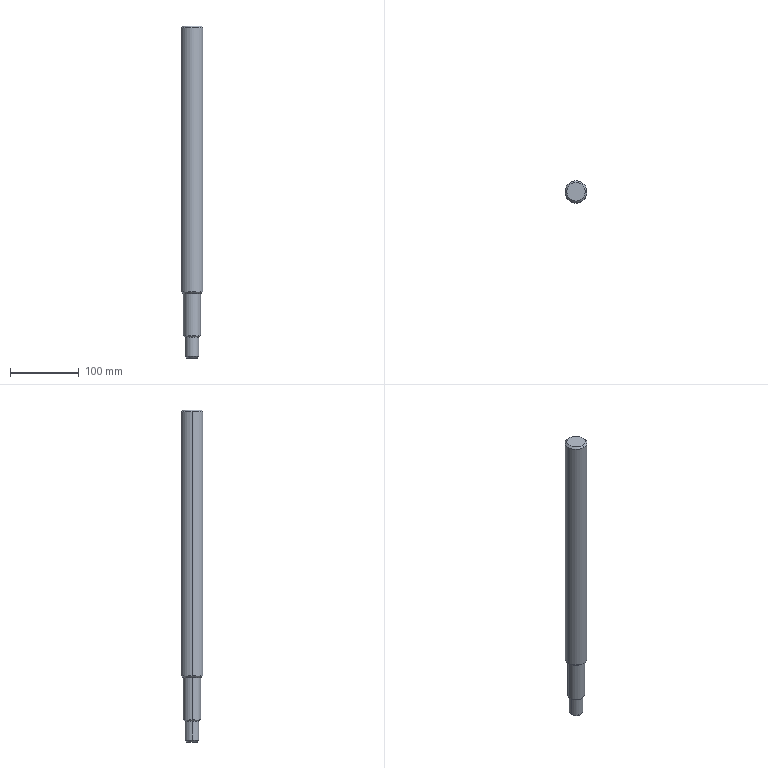Part | SolidWorks | features BaseBody 1 | 1 solid | 17 faces | box 32 x 32 x 484 mm | volume 353493 mm3 | cone 8 | cylinder 6 | plane 3 | commonest cylinder face diameters 20 x2 25 x2 32 x2
STEP:
#1=CARTESIAN_POINT('',(0.,16.,481.5));
#2=VERTEX_POINT('',#1);
#3=CARTESIAN_POINT('',(16.,0.,481.5));
#4=VERTEX_POINT('',#3);
#5=CARTESIAN_POINT('',(0.,0.,481.5));
#6=DIRECTION('',(0.,0.,-1.));
#7=DIRECTION('',(-1.,0.,0.));
#8=AXIS2_PLACEMENT_3D('',#5,#6,#7);
#9=CIRCLE('',#8,16.);
#10=EDGE_CURVE('',#2,#4,#9,.T.);
#11=ORIENTED_EDGE('',*,*,#10,.T.);
#12=CARTESIAN_POINT('',(16.,0.,96.5));
#13=VERTEX_POINT('',#12);
#14=CARTESIAN_POINT('',(16.,0.,484.));
#15=DIRECTION('',(0.,0.,-1.));
#16=VECTOR('',#15,1000.);
#17=LINE('',#14,#16);
#18=EDGE_CURVE('',#4,#13,#17,.T.);
#19=ORIENTED_EDGE('',*,*,#18,.T.);
#20=CARTESIAN_POINT('',(0.,16.,96.5));
#21=VERTEX_POINT('',#20);
#22=CARTESIAN_POINT('',(0.,0.,96.5));
#23=DIRECTION('',(0.,0.,1.));
#24=DIRECTION('',(-1.,0.,0.));
#25=AXIS2_PLACEMENT_3D('',#22,#23,#24);
#26=CIRCLE('',#25,16.);
#27=EDGE_CURVE('',#13,#21,#26,.T.);
#28=ORIENTED_EDGE('',*,*,#27,.T.);
#29=CARTESIAN_POINT('',(-16.,0.,96.5));
#30=VERTEX_POINT('',#29);
#31=CARTESIAN_POINT('',(0.,0.,96.5));
#32=DIRECTION('',(0.,0.,1.));
#33=DIRECTION('',(-1.,0.,0.));
#34=AXIS2_PLACEMENT_3D('',#31,#32,#33);
#35=CIRCLE('',#34,16.);
#36=EDGE_CURVE('',#21,#30,#35,.T.);
#37=ORIENTED_EDGE('',*,*,#36,.T.);
#38=CARTESIAN_POINT('',(-16.,0.,481.5));
#39=VERTEX_POINT('',#38);
#40=CARTESIAN_POINT('',(-16.,0.,484.));
#41=DIRECTION('',(0.,0.,-1.));
#42=VECTOR('',#41,1000.);
#43=LINE('',#40,#42);
#44=EDGE_CURVE('',#39,#30,#43,.T.);
#45=ORIENTED_EDGE('',*,*,#44,.F.);
#46=CARTESIAN_POINT('',(0.,0.,481.5));
#47=DIRECTION('',(0.,0.,-1.));
#48=DIRECTION('',(-1.,0.,0.));
#49=AXIS2_PLACEMENT_3D('',#46,#47,#48);
#50=CIRCLE('',#49,16.);
#51=EDGE_CURVE('',#39,#2,#50,.T.);
#52=ORIENTED_EDGE('',*,*,#51,.T.);
#53=EDGE_LOOP('',(#11,#19,#28,#37,#45,#52));
#54=FACE_OUTER_BOUND('',#53,.T.);
#55=CARTESIAN_POINT('',(0.,0.,484.));
#56=DIRECTION('',(0.,0.,-1.));
#57=DIRECTION('',(-1.,0.,0.));
#58=AXIS2_PLACEMENT_3D('',#55,#56,#57);
#59=CYLINDRICAL_SURFACE('',#58,16.);
#60=ADVANCED_FACE('',(#54),#59,.T.);
#61=CARTESIAN_POINT('',(0.,-13.5,94.));
#62=VERTEX_POINT('',#61);
#63=CARTESIAN_POINT('',(0.,13.5,94.));
#64=VERTEX_POINT('',#63);
#65=CARTESIAN_POINT('',(0.,0.,94.));
#66=DIRECTION('',(0.,0.,1.));
#67=DIRECTION('',(0.,-1.,0.));
#68=AXIS2_PLACEMENT_3D('',#65,#66,#67);
#69=CIRCLE('',#68,13.5);
#70=EDGE_CURVE('',#62,#64,#69,.T.);
#71=ORIENTED_EDGE('',*,*,#70,.T.);
#72=CARTESIAN_POINT('',(0.,16.,96.5));
#73=DIRECTION('',(0.,0.7071,0.7071));
#74=VECTOR('',#73,1000.);
#75=LINE('',#72,#74);
#76=EDGE_CURVE('',#64,#21,#75,.T.);
#77=ORIENTED_EDGE('',*,*,#76,.T.);
#78=ORIENTED_EDGE('',*,*,#27,.F.);
#79=CARTESIAN_POINT('',(0.,-16.,96.5));
#80=VERTEX_POINT('',#79);
#81=CARTESIAN_POINT('',(0.,0.,96.5));
#82=DIRECTION('',(0.,0.,1.));
#83=DIRECTION('',(-1.,0.,0.));
#84=AXIS2_PLACEMENT_3D('',#81,#82,#83);
#85=CIRCLE('',#84,16.);
#86=EDGE_CURVE('',#80,#13,#85,.T.);
#87=ORIENTED_EDGE('',*,*,#86,.F.);
#88=CARTESIAN_POINT('',(0.,-16.,96.5));
#89=DIRECTION('',(0.,-0.7071,0.7071));
#90=VECTOR('',#89,1000.);
#91=LINE('',#88,#90);
#92=EDGE_CURVE('',#62,#80,#91,.T.);
#93=ORIENTED_EDGE('',*,*,#92,.F.);
#94=EDGE_LOOP('',(#71,#77,#78,#87,#93));
#95=FACE_OUTER_BOUND('',#94,.T.);
#96=CARTESIAN_POINT('',(0.,0.,96.5));
#97=DIRECTION('',(0.,0.,1.));
#98=DIRECTION('',(0.,-1.,0.));
#99=AXIS2_PLACEMENT_3D('',#96,#97,#98);
#100=CONICAL_SURFACE('',#99,16.,0.7854);
#101=ADVANCED_FACE('',(#95),#100,.T.);
#102=CARTESIAN_POINT('',(0.,13.5,484.));
#103=VERTEX_POINT('',#102);
#104=CARTESIAN_POINT('',(0.,-13.5,484.));
#105=VERTEX_POINT('',#104);
#106=CARTESIAN_POINT('',(0.,0.,484.));
#107=DIRECTION('',(0.,0.,-1.));
#108=DIRECTION('',(0.,1.,0.));
#109=AXIS2_PLACEMENT_3D('',#106,#107,#108);
#110=CIRCLE('',#109,13.5);
#111=EDGE_CURVE('',#103,#105,#110,.T.);
#112=ORIENTED_EDGE('',*,*,#111,.T.);
#113=CARTESIAN_POINT('',(0.,-16.,481.5));
#114=VERTEX_POINT('',#113);
#115=CARTESIAN_POINT('',(0.,-16.,481.5));
#116=DIRECTION('',(0.,-0.7071,-0.7071));
#117=VECTOR('',#116,1000.);
#118=LINE('',#115,#117);
#119=EDGE_CURVE('',#105,#114,#118,.T.);
#120=ORIENTED_EDGE('',*,*,#119,.T.);
#121=CARTESIAN_POINT('',(0.,0.,481.5));
#122=DIRECTION('',(0.,0.,-1.));
#123=DIRECTION('',(-1.,0.,0.));
#124=AXIS2_PLACEMENT_3D('',#121,#122,#123);
#125=CIRCLE('',#124,16.);
#126=EDGE_CURVE('',#4,#114,#125,.T.);
#127=ORIENTED_EDGE('',*,*,#126,.F.);
#128=ORIENTED_EDGE('',*,*,#10,.F.);
#129=CARTESIAN_POINT('',(0.,16.,481.5));
#130=DIRECTION('',(0.,0.7071,-0.7071));
#131=VECTOR('',#130,1000.);
#132=LINE('',#129,#131);
#133=EDGE_CURVE('',#103,#2,#132,.T.);
#134=ORIENTED_EDGE('',*,*,#133,.F.);
#135=EDGE_LOOP('',(#112,#120,#127,#128,#134));
#136=FACE_OUTER_BOUND('',#135,.T.);
#137=CARTESIAN_POINT('',(0.,0.,481.5));
#138=DIRECTION('',(0.,0.,-1.));
#139=DIRECTION('',(0.,1.,0.));
#140=AXIS2_PLACEMENT_3D('',#137,#138,#139);
#141=CONICAL_SURFACE('',#140,16.,0.7854);
#142=ADVANCED_FACE('',(#136),#141,.T.);
#143=CARTESIAN_POINT('',(-12.5,0.,94.));
#144=VERTEX_POINT('',#143);
#145=CARTESIAN_POINT('',(12.5,0.,94.));
#146=VERTEX_POINT('',#145);
#147=CARTESIAN_POINT('',(0.,0.,94.));
#148=DIRECTION('',(0.,0.,-1.));
#149=DIRECTION('',(-1.,0.,0.));
#150=AXIS2_PLACEMENT_3D('',#147,#148,#149);
#151=CIRCLE('',#150,12.5);
#152=EDGE_CURVE('',#144,#146,#151,.T.);
#153=ORIENTED_EDGE('',*,*,#152,.T.);
#154=CARTESIAN_POINT('',(12.5,0.,32.5));
#155=VERTEX_POINT('',#154);
#156=CARTESIAN_POINT('',(12.5,0.,94.));
#157=DIRECTION('',(0.,0.,-1.));
#158=VECTOR('',#157,1000.);
#159=LINE('',#156,#158);
#160=EDGE_CURVE('',#146,#155,#159,.T.);
#161=ORIENTED_EDGE('',*,*,#160,.T.);
#162=CARTESIAN_POINT('',(-12.5,0.,32.5));
#163=VERTEX_POINT('',#162);
#164=CARTESIAN_POINT('',(0.,0.,32.5));
#165=DIRECTION('',(0.,0.,1.));
#166=DIRECTION('',(-1.,0.,0.));
#167=AXIS2_PLACEMENT_3D('',#164,#165,#166);
#168=CIRCLE('',#167,12.5);
#169=EDGE_CURVE('',#155,#163,#168,.T.);
#170=ORIENTED_EDGE('',*,*,#169,.T.);
#171=CARTESIAN_POINT('',(-12.5,0.,94.));
#172=DIRECTION('',(0.,0.,-1.));
#173=VECTOR('',#172,1000.);
#174=LINE('',#171,#173);
#175=EDGE_CURVE('',#144,#163,#174,.T.);
#176=ORIENTED_EDGE('',*,*,#175,.F.);
#177=EDGE_LOOP('',(#153,#161,#170,#176));
#178=FACE_OUTER_BOUND('',#177,.T.);
#179=CARTESIAN_POINT('',(0.,0.,94.));
#180=DIRECTION('',(0.,0.,-1.));
#181=DIRECTION('',(-1.,0.,0.));
#182=AXIS2_PLACEMENT_3D('',#179,#180,#181);
#183=CYLINDRICAL_SURFACE('',#182,12.5);
#184=ADVANCED_FACE('',(#178),#183,.T.);
#185=CARTESIAN_POINT('',(10.,0.,30.));
#186=VERTEX_POINT('',#185);
#187=CARTESIAN_POINT('',(-10.,0.,30.));
#188=VERTEX_POINT('',#187);
#189=CARTESIAN_POINT('',(0.,0.,30.));
#190=DIRECTION('',(0.,0.,1.));
#191=DIRECTION('',(-1.,0.,0.));
#192=AXIS2_PLACEMENT_3D('',#189,#190,#191);
#193=CIRCLE('',#192,10.);
#194=EDGE_CURVE('',#186,#188,#193,.T.);
#195=ORIENTED_EDGE('',*,*,#194,.T.);
#196=CARTESIAN_POINT('',(-12.5,0.,32.5));
#197=DIRECTION('',(-0.7071,0.,0.7071));
#198=VECTOR('',#197,1000.);
#199=LINE('',#196,#198);
#200=EDGE_CURVE('',#188,#163,#199,.T.);
#201=ORIENTED_EDGE('',*,*,#200,.T.);
#202=ORIENTED_EDGE('',*,*,#169,.F.);
#203=CARTESIAN_POINT('',(12.5,0.,32.5));
#204=DIRECTION('',(0.7071,0.,0.7071));
#205=VECTOR('',#204,1000.);
#206=LINE('',#203,#205);
#207=EDGE_CURVE('',#186,#155,#206,.T.);
#208=ORIENTED_EDGE('',*,*,#207,.F.);
#209=EDGE_LOOP('',(#195,#201,#202,#208));
#210=FACE_OUTER_BOUND('',#209,.T.);
#211=CARTESIAN_POINT('',(0.,0.,32.5));
#212=DIRECTION('',(0.,0.,1.));
#213=DIRECTION('',(1.,0.,0.));
#214=AXIS2_PLACEMENT_3D('',#211,#212,#213);
#215=CONICAL_SURFACE('',#214,12.5,0.7854);
#216=ADVANCED_FACE('',(#210),#215,.T.);
#217=ORIENTED_EDGE('',*,*,#194,.F.);
#218=CARTESIAN_POINT('',(10.,0.,2.5));
#219=VERTEX_POINT('',#218);
#220=CARTESIAN_POINT('',(10.,0.,30.));
#221=DIRECTION('',(0.,0.,-1.));
#222=VECTOR('',#221,1000.);
#223=LINE('',#220,#222);
#224=EDGE_CURVE('',#186,#219,#223,.T.);
#225=ORIENTED_EDGE('',*,*,#224,.T.);
#226=CARTESIAN_POINT('',(-10.,0.,2.5));
#227=VERTEX_POINT('',#226);
#228=CARTESIAN_POINT('',(0.,0.,2.5));
#229=DIRECTION('',(0.,0.,1.));
#230=DIRECTION('',(-1.,0.,0.));
#231=AXIS2_PLACEMENT_3D('',#228,#229,#230);
#232=CIRCLE('',#231,10.);
#233=EDGE_CURVE('',#219,#227,#232,.T.);
#234=ORIENTED_EDGE('',*,*,#233,.T.);
#235=CARTESIAN_POINT('',(-10.,0.,30.));
#236=DIRECTION('',(0.,0.,-1.));
#237=VECTOR('',#236,1000.);
#238=LINE('',#235,#237);
#239=EDGE_CURVE('',#188,#227,#238,.T.);
#240=ORIENTED_EDGE('',*,*,#239,.F.);
#241=EDGE_LOOP('',(#217,#225,#234,#240));
#242=FACE_OUTER_BOUND('',#241,.T.);
#243=CARTESIAN_POINT('',(0.,0.,30.));
#244=DIRECTION('',(0.,0.,-1.));
#245=DIRECTION('',(-1.,0.,0.));
#246=AXIS2_PLACEMENT_3D('',#243,#244,#245);
#247=CYLINDRICAL_SURFACE('',#246,10.);
#248=ADVANCED_FACE('',(#242),#247,.T.);
#249=CARTESIAN_POINT('',(7.5,0.,0.));
#250=VERTEX_POINT('',#249);
#251=CARTESIAN_POINT('',(-7.5,0.,0.));
#252=VERTEX_POINT('',#251);
#253=CARTESIAN_POINT('',(0.,0.,0.));
#254=DIRECTION('',(0.,0.,1.));
#255=DIRECTION('',(1.,0.,0.));
#256=AXIS2_PLACEMENT_3D('',#253,#254,#255);
#257=CIRCLE('',#256,7.5);
#258=EDGE_CURVE('',#250,#252,#257,.T.);
#259=ORIENTED_EDGE('',*,*,#258,.T.);
#260=CARTESIAN_POINT('',(-10.,0.,2.5));
#261=DIRECTION('',(-0.7071,0.,0.7071));
#262=VECTOR('',#261,1000.);
#263=LINE('',#260,#262);
#264=EDGE_CURVE('',#252,#227,#263,.T.);
#265=ORIENTED_EDGE('',*,*,#264,.T.);
#266=ORIENTED_EDGE('',*,*,#233,.F.);
#267=CARTESIAN_POINT('',(10.,0.,2.5));
#268=DIRECTION('',(0.7071,0.,0.7071));
#269=VECTOR('',#268,1000.);
#270=LINE('',#267,#269);
#271=EDGE_CURVE('',#250,#219,#270,.T.);
#272=ORIENTED_EDGE('',*,*,#271,.F.);
#273=EDGE_LOOP('',(#259,#265,#266,#272));
#274=FACE_OUTER_BOUND('',#273,.T.);
#275=CARTESIAN_POINT('',(0.,0.,2.5));
#276=DIRECTION('',(0.,0.,1.));
#277=DIRECTION('',(1.,0.,0.));
#278=AXIS2_PLACEMENT_3D('',#275,#276,#277);
#279=CONICAL_SURFACE('',#278,10.,0.7854);
#280=ADVANCED_FACE('',(#274),#279,.T.);
#281=ORIENTED_EDGE('',*,*,#18,.F.);
#282=ORIENTED_EDGE('',*,*,#126,.T.);
#283=CARTESIAN_POINT('',(0.,0.,481.5));
#284=DIRECTION('',(0.,0.,-1.));
#285=DIRECTION('',(-1.,0.,0.));
#286=AXIS2_PLACEMENT_3D('',#283,#284,#285);
#287=CIRCLE('',#286,16.);
#288=EDGE_CURVE('',#114,#39,#287,.T.);
#289=ORIENTED_EDGE('',*,*,#288,.T.);
#290=ORIENTED_EDGE('',*,*,#44,.T.);
#291=CARTESIAN_POINT('',(0.,0.,96.5));
#292=DIRECTION('',(0.,0.,1.));
#293=DIRECTION('',(-1.,0.,0.));
#294=AXIS2_PLACEMENT_3D('',#291,#292,#293);
#295=CIRCLE('',#294,16.);
#296=EDGE_CURVE('',#30,#80,#295,.T.);
#297=ORIENTED_EDGE('',*,*,#296,.T.);
#298=ORIENTED_EDGE('',*,*,#86,.T.);
#299=EDGE_LOOP('',(#281,#282,#289,#290,#297,#298));
#300=FACE_OUTER_BOUND('',#299,.T.);
#301=CARTESIAN_POINT('',(0.,0.,484.));
#302=DIRECTION('',(0.,0.,-1.));
#303=DIRECTION('',(-1.,0.,0.));
#304=AXIS2_PLACEMENT_3D('',#301,#302,#303);
#305=CYLINDRICAL_SURFACE('',#304,16.);
#306=ADVANCED_FACE('',(#300),#305,.T.);
#307=ORIENTED_EDGE('',*,*,#76,.F.);
#308=CARTESIAN_POINT('',(0.,0.,94.));
#309=DIRECTION('',(0.,0.,1.));
#310=DIRECTION('',(0.,-1.,0.));
#311=AXIS2_PLACEMENT_3D('',#308,#309,#310);
#312=CIRCLE('',#311,13.5);
#313=EDGE_CURVE('',#64,#62,#312,.T.);
#314=ORIENTED_EDGE('',*,*,#313,.T.);
#315=ORIENTED_EDGE('',*,*,#92,.T.);
#316=ORIENTED_EDGE('',*,*,#296,.F.);
#317=ORIENTED_EDGE('',*,*,#36,.F.);
#318=EDGE_LOOP('',(#307,#314,#315,#316,#317));
#319=FACE_OUTER_BOUND('',#318,.T.);
#320=CARTESIAN_POINT('',(0.,0.,96.5));
#321=DIRECTION('',(0.,0.,1.));
#322=DIRECTION('',(0.,-1.,0.));
#323=AXIS2_PLACEMENT_3D('',#320,#321,#322);
#324=CONICAL_SURFACE('',#323,16.,0.7854);
#325=ADVANCED_FACE('',(#319),#324,.T.);
#326=ORIENTED_EDGE('',*,*,#119,.F.);
#327=CARTESIAN_POINT('',(0.,0.,484.));
#328=DIRECTION('',(0.,0.,-1.));
#329=DIRECTION('',(0.,1.,0.));
#330=AXIS2_PLACEMENT_3D('',#327,#328,#329);
#331=CIRCLE('',#330,13.5);
#332=EDGE_CURVE('',#105,#103,#331,.T.);
#333=ORIENTED_EDGE('',*,*,#332,.T.);
#334=ORIENTED_EDGE('',*,*,#133,.T.);
#335=ORIENTED_EDGE('',*,*,#51,.F.);
#336=ORIENTED_EDGE('',*,*,#288,.F.);
#337=EDGE_LOOP('',(#326,#333,#334,#335,#336));
#338=FACE_OUTER_BOUND('',#337,.T.);
#339=CARTESIAN_POINT('',(0.,0.,481.5));
#340=DIRECTION('',(0.,0.,-1.));
#341=DIRECTION('',(0.,1.,0.));
#342=AXIS2_PLACEMENT_3D('',#339,#340,#341);
#343=CONICAL_SURFACE('',#342,16.,0.7854);
#344=ADVANCED_FACE('',(#338),#343,.T.);
#345=ORIENTED_EDGE('',*,*,#152,.F.);
#346=CARTESIAN_POINT('',(0.,0.,94.));
#347=DIRECTION('',(0.,0.,-1.));
#348=DIRECTION('',(-1.,0.,0.));
#349=AXIS2_PLACEMENT_3D('',#346,#347,#348);
#350=CIRCLE('',#349,12.5);
#351=EDGE_CURVE('',#146,#144,#350,.T.);
#352=ORIENTED_EDGE('',*,*,#351,.F.);
#353=EDGE_LOOP('',(#345,#352));
#354=FACE_BOUND('',#353,.T.);
#355=ORIENTED_EDGE('',*,*,#70,.F.);
#356=ORIENTED_EDGE('',*,*,#313,.F.);
#357=EDGE_LOOP('',(#355,#356));
#358=FACE_OUTER_BOUND('',#357,.T.);
#359=CARTESIAN_POINT('',(0.,0.,94.));
#360=DIRECTION('',(0.,0.,1.));
#361=DIRECTION('',(1.,0.,0.));
#362=AXIS2_PLACEMENT_3D('',#359,#360,#361);
#363=PLANE('',#362);
#364=ADVANCED_FACE('',(#354,#358),#363,.F.);
#365=ORIENTED_EDGE('',*,*,#111,.F.);
#366=ORIENTED_EDGE('',*,*,#332,.F.);
#367=EDGE_LOOP('',(#365,#366));
#368=FACE_OUTER_BOUND('',#367,.T.);
#369=CARTESIAN_POINT('',(0.,0.,484.));
#370=DIRECTION('',(0.,0.,1.));
#371=DIRECTION('',(1.,0.,0.));
#372=AXIS2_PLACEMENT_3D('',#369,#370,#371);
#373=PLANE('',#372);
#374=ADVANCED_FACE('',(#368),#373,.T.);
#375=ORIENTED_EDGE('',*,*,#160,.F.);
#376=ORIENTED_EDGE('',*,*,#351,.T.);
#377=ORIENTED_EDGE('',*,*,#175,.T.);
#378=CARTESIAN_POINT('',(0.,0.,32.5));
#379=DIRECTION('',(0.,0.,1.));
#380=DIRECTION('',(-1.,0.,0.));
#381=AXIS2_PLACEMENT_3D('',#378,#379,#380);
#382=CIRCLE('',#381,12.5);
#383=EDGE_CURVE('',#163,#155,#382,.T.);
#384=ORIENTED_EDGE('',*,*,#383,.T.);
#385=EDGE_LOOP('',(#375,#376,#377,#384));
#386=FACE_OUTER_BOUND('',#385,.T.);
#387=CARTESIAN_POINT('',(0.,0.,94.));
#388=DIRECTION('',(0.,0.,-1.));
#389=DIRECTION('',(-1.,0.,0.));
#390=AXIS2_PLACEMENT_3D('',#387,#388,#389);
#391=CYLINDRICAL_SURFACE('',#390,12.5);
#392=ADVANCED_FACE('',(#386),#391,.T.);
#393=ORIENTED_EDGE('',*,*,#200,.F.);
#394=CARTESIAN_POINT('',(0.,0.,30.));
#395=DIRECTION('',(0.,0.,1.));
#396=DIRECTION('',(-1.,0.,0.));
#397=AXIS2_PLACEMENT_3D('',#394,#395,#396);
#398=CIRCLE('',#397,10.);
#399=EDGE_CURVE('',#188,#186,#398,.T.);
#400=ORIENTED_EDGE('',*,*,#399,.T.);
#401=ORIENTED_EDGE('',*,*,#207,.T.);
#402=ORIENTED_EDGE('',*,*,#383,.F.);
#403=EDGE_LOOP('',(#393,#400,#401,#402));
#404=FACE_OUTER_BOUND('',#403,.T.);
#405=CARTESIAN_POINT('',(0.,0.,32.5));
#406=DIRECTION('',(0.,0.,1.));
#407=DIRECTION('',(1.,0.,0.));
#408=AXIS2_PLACEMENT_3D('',#405,#406,#407);
#409=CONICAL_SURFACE('',#408,12.5,0.7854);
#410=ADVANCED_FACE('',(#404),#409,.T.);
#411=ORIENTED_EDGE('',*,*,#224,.F.);
#412=ORIENTED_EDGE('',*,*,#399,.F.);
#413=ORIENTED_EDGE('',*,*,#239,.T.);
#414=CARTESIAN_POINT('',(0.,0.,2.5));
#415=DIRECTION('',(0.,0.,1.));
#416=DIRECTION('',(-1.,0.,0.));
#417=AXIS2_PLACEMENT_3D('',#414,#415,#416);
#418=CIRCLE('',#417,10.);
#419=EDGE_CURVE('',#227,#219,#418,.T.);
#420=ORIENTED_EDGE('',*,*,#419,.T.);
#421=EDGE_LOOP('',(#411,#412,#413,#420));
#422=FACE_OUTER_BOUND('',#421,.T.);
#423=CARTESIAN_POINT('',(0.,0.,30.));
#424=DIRECTION('',(0.,0.,-1.));
#425=DIRECTION('',(-1.,0.,0.));
#426=AXIS2_PLACEMENT_3D('',#423,#424,#425);
#427=CYLINDRICAL_SURFACE('',#426,10.);
#428=ADVANCED_FACE('',(#422),#427,.T.);
#429=ORIENTED_EDGE('',*,*,#264,.F.);
#430=CARTESIAN_POINT('',(0.,0.,0.));
#431=DIRECTION('',(0.,0.,1.));
#432=DIRECTION('',(1.,0.,0.));
#433=AXIS2_PLACEMENT_3D('',#430,#431,#432);
#434=CIRCLE('',#433,7.5);
#435=EDGE_CURVE('',#252,#250,#434,.T.);
#436=ORIENTED_EDGE('',*,*,#435,.T.);
#437=ORIENTED_EDGE('',*,*,#271,.T.);
#438=ORIENTED_EDGE('',*,*,#419,.F.);
#439=EDGE_LOOP('',(#429,#436,#437,#438));
#440=FACE_OUTER_BOUND('',#439,.T.);
#441=CARTESIAN_POINT('',(0.,0.,2.5));
#442=DIRECTION('',(0.,0.,1.));
#443=DIRECTION('',(1.,0.,0.));
#444=AXIS2_PLACEMENT_3D('',#441,#442,#443);
#445=CONICAL_SURFACE('',#444,10.,0.7854);
#446=ADVANCED_FACE('',(#440),#445,.T.);
#447=ORIENTED_EDGE('',*,*,#258,.F.);
#448=ORIENTED_EDGE('',*,*,#435,.F.);
#449=EDGE_LOOP('',(#447,#448));
#450=FACE_OUTER_BOUND('',#449,.T.);
#451=CARTESIAN_POINT('',(0.,0.,0.));
#452=DIRECTION('',(0.,0.,1.));
#453=DIRECTION('',(1.,0.,0.));
#454=AXIS2_PLACEMENT_3D('',#451,#452,#453);
#455=PLANE('',#454);
#456=ADVANCED_FACE('',(#450),#455,.F.);
#457=CLOSED_SHELL('',(#60,#101,#142,#184,#216,#248,#280,#306,#325,#344,#364,#374,#392,#410,#428,#446,#456));
#458=MANIFOLD_SOLID_BREP('',#457);
#459=CARTESIAN_POINT('',(0.,0.,0.));
#460=DIRECTION('',(0.,0.,1.));
#461=DIRECTION('',(1.,0.,0.));
#462=AXIS2_PLACEMENT_3D('',#459,#460,#461);
#463=(LENGTH_UNIT()NAMED_UNIT(*)SI_UNIT(.MILLI.,.METRE.));
#464=UNCERTAINTY_MEASURE_WITH_UNIT(LENGTH_MEASURE(0.00001),#463,'','');
#465=(NAMED_UNIT(*)PLANE_ANGLE_UNIT()SI_UNIT($,.RADIAN.));
#466=(NAMED_UNIT(*)SI_UNIT($,.STERADIAN.)SOLID_ANGLE_UNIT());
#467=(GEOMETRIC_REPRESENTATION_CONTEXT(3)GLOBAL_UNCERTAINTY_ASSIGNED_CONTEXT((#464))GLOBAL_UNIT_ASSIGNED_CONTEXT((#463,#465,#466))REPRESENTATION_CONTEXT('',''));
#468=ADVANCED_BREP_SHAPE_REPRESENTATION('',(#458,#462),#467);